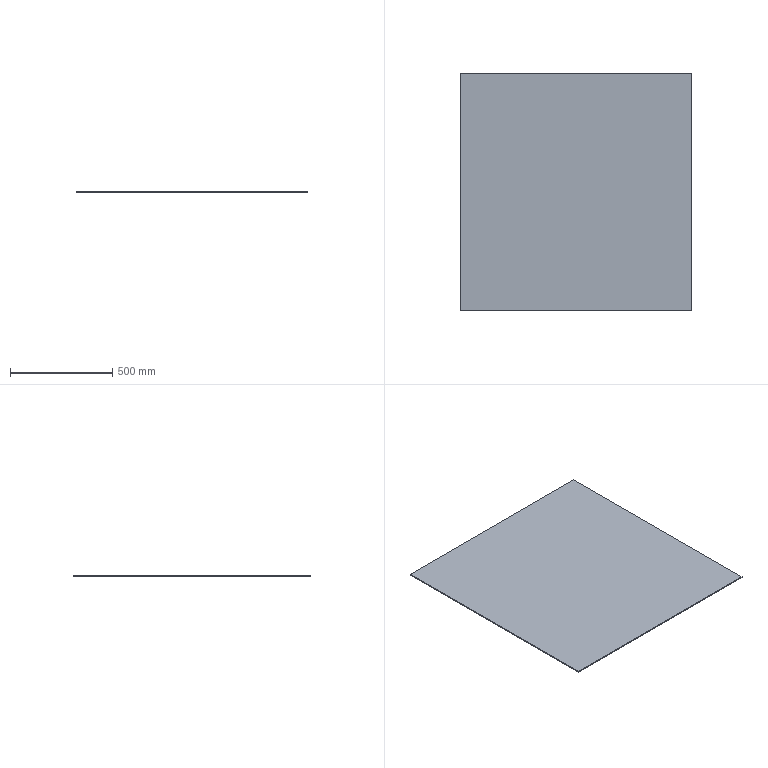Part | 1 solid | 6 faces | box 1135 x 1165 x 5 mm | volume 6611375 mm3 | plane 6
STEP:
#1=CARTESIAN_POINT('',(567.5,-582.5,0.));
#2=VERTEX_POINT('',#1);
#3=CARTESIAN_POINT('',(567.5,582.5,0.));
#4=VERTEX_POINT('',#3);
#5=CARTESIAN_POINT('',(567.5,582.5,0.));
#6=DIRECTION('',(0.,1.,0.));
#7=VECTOR('',#6,1000.);
#8=LINE('',#5,#7);
#9=EDGE_CURVE('',#2,#4,#8,.T.);
#10=ORIENTED_EDGE('',*,*,#9,.T.);
#11=CARTESIAN_POINT('',(567.5,582.5,5.));
#12=VERTEX_POINT('',#11);
#13=CARTESIAN_POINT('',(567.5,582.5,5.));
#14=DIRECTION('',(0.,0.,-1.));
#15=VECTOR('',#14,1000.);
#16=LINE('',#13,#15);
#17=EDGE_CURVE('',#12,#4,#16,.T.);
#18=ORIENTED_EDGE('',*,*,#17,.F.);
#19=CARTESIAN_POINT('',(567.5,-582.5,5.));
#20=VERTEX_POINT('',#19);
#21=CARTESIAN_POINT('',(567.5,582.5,5.));
#22=DIRECTION('',(0.,1.,0.));
#23=VECTOR('',#22,1000.);
#24=LINE('',#21,#23);
#25=EDGE_CURVE('',#20,#12,#24,.T.);
#26=ORIENTED_EDGE('',*,*,#25,.F.);
#27=CARTESIAN_POINT('',(567.5,-582.5,5.));
#28=DIRECTION('',(0.,0.,-1.));
#29=VECTOR('',#28,1000.);
#30=LINE('',#27,#29);
#31=EDGE_CURVE('',#20,#2,#30,.T.);
#32=ORIENTED_EDGE('',*,*,#31,.T.);
#33=EDGE_LOOP('',(#10,#18,#26,#32));
#34=FACE_OUTER_BOUND('',#33,.T.);
#35=CARTESIAN_POINT('',(567.5,582.5,5.));
#36=DIRECTION('',(-1.,0.,0.));
#37=DIRECTION('',(0.,-1.,0.));
#38=AXIS2_PLACEMENT_3D('',#35,#36,#37);
#39=PLANE('',#38);
#40=ADVANCED_FACE('',(#34),#39,.F.);
#41=CARTESIAN_POINT('',(-567.5,582.5,0.));
#42=VERTEX_POINT('',#41);
#43=CARTESIAN_POINT('',(-567.5,582.5,0.));
#44=DIRECTION('',(-1.,0.,0.));
#45=VECTOR('',#44,1000.);
#46=LINE('',#43,#45);
#47=EDGE_CURVE('',#4,#42,#46,.T.);
#48=ORIENTED_EDGE('',*,*,#47,.T.);
#49=CARTESIAN_POINT('',(-567.5,582.5,5.));
#50=VERTEX_POINT('',#49);
#51=CARTESIAN_POINT('',(-567.5,582.5,5.));
#52=DIRECTION('',(0.,0.,-1.));
#53=VECTOR('',#52,1000.);
#54=LINE('',#51,#53);
#55=EDGE_CURVE('',#50,#42,#54,.T.);
#56=ORIENTED_EDGE('',*,*,#55,.F.);
#57=CARTESIAN_POINT('',(-567.5,582.5,5.));
#58=DIRECTION('',(-1.,0.,0.));
#59=VECTOR('',#58,1000.);
#60=LINE('',#57,#59);
#61=EDGE_CURVE('',#12,#50,#60,.T.);
#62=ORIENTED_EDGE('',*,*,#61,.F.);
#63=ORIENTED_EDGE('',*,*,#17,.T.);
#64=EDGE_LOOP('',(#48,#56,#62,#63));
#65=FACE_OUTER_BOUND('',#64,.T.);
#66=CARTESIAN_POINT('',(-567.5,582.5,5.));
#67=DIRECTION('',(0.,-1.,0.));
#68=DIRECTION('',(0.,0.,-1.));
#69=AXIS2_PLACEMENT_3D('',#66,#67,#68);
#70=PLANE('',#69);
#71=ADVANCED_FACE('',(#65),#70,.F.);
#72=CARTESIAN_POINT('',(-567.5,-582.5,0.));
#73=VERTEX_POINT('',#72);
#74=CARTESIAN_POINT('',(-567.5,582.5,0.));
#75=DIRECTION('',(0.,-1.,0.));
#76=VECTOR('',#75,1000.);
#77=LINE('',#74,#76);
#78=EDGE_CURVE('',#42,#73,#77,.T.);
#79=ORIENTED_EDGE('',*,*,#78,.T.);
#80=CARTESIAN_POINT('',(-567.5,-582.5,5.));
#81=VERTEX_POINT('',#80);
#82=CARTESIAN_POINT('',(-567.5,-582.5,5.));
#83=DIRECTION('',(0.,0.,-1.));
#84=VECTOR('',#83,1000.);
#85=LINE('',#82,#84);
#86=EDGE_CURVE('',#81,#73,#85,.T.);
#87=ORIENTED_EDGE('',*,*,#86,.F.);
#88=CARTESIAN_POINT('',(-567.5,582.5,5.));
#89=DIRECTION('',(0.,-1.,0.));
#90=VECTOR('',#89,1000.);
#91=LINE('',#88,#90);
#92=EDGE_CURVE('',#50,#81,#91,.T.);
#93=ORIENTED_EDGE('',*,*,#92,.F.);
#94=ORIENTED_EDGE('',*,*,#55,.T.);
#95=EDGE_LOOP('',(#79,#87,#93,#94));
#96=FACE_OUTER_BOUND('',#95,.T.);
#97=CARTESIAN_POINT('',(-567.5,582.5,5.));
#98=DIRECTION('',(1.,0.,0.));
#99=DIRECTION('',(0.,1.,0.));
#100=AXIS2_PLACEMENT_3D('',#97,#98,#99);
#101=PLANE('',#100);
#102=ADVANCED_FACE('',(#96),#101,.F.);
#103=CARTESIAN_POINT('',(-567.5,-582.5,0.));
#104=DIRECTION('',(1.,0.,0.));
#105=VECTOR('',#104,1000.);
#106=LINE('',#103,#105);
#107=EDGE_CURVE('',#73,#2,#106,.T.);
#108=ORIENTED_EDGE('',*,*,#107,.T.);
#109=ORIENTED_EDGE('',*,*,#31,.F.);
#110=CARTESIAN_POINT('',(-567.5,-582.5,5.));
#111=DIRECTION('',(1.,0.,0.));
#112=VECTOR('',#111,1000.);
#113=LINE('',#110,#112);
#114=EDGE_CURVE('',#81,#20,#113,.T.);
#115=ORIENTED_EDGE('',*,*,#114,.F.);
#116=ORIENTED_EDGE('',*,*,#86,.T.);
#117=EDGE_LOOP('',(#108,#109,#115,#116));
#118=FACE_OUTER_BOUND('',#117,.T.);
#119=CARTESIAN_POINT('',(-567.5,-582.5,5.));
#120=DIRECTION('',(0.,1.,0.));
#121=DIRECTION('',(0.,0.,1.));
#122=AXIS2_PLACEMENT_3D('',#119,#120,#121);
#123=PLANE('',#122);
#124=ADVANCED_FACE('',(#118),#123,.F.);
#125=ORIENTED_EDGE('',*,*,#25,.T.);
#126=ORIENTED_EDGE('',*,*,#61,.T.);
#127=ORIENTED_EDGE('',*,*,#92,.T.);
#128=ORIENTED_EDGE('',*,*,#114,.T.);
#129=EDGE_LOOP('',(#125,#126,#127,#128));
#130=FACE_OUTER_BOUND('',#129,.T.);
#131=CARTESIAN_POINT('',(0.,0.,5.));
#132=DIRECTION('',(0.,0.,1.));
#133=DIRECTION('',(1.,0.,0.));
#134=AXIS2_PLACEMENT_3D('',#131,#132,#133);
#135=PLANE('',#134);
#136=ADVANCED_FACE('',(#130),#135,.T.);
#137=ORIENTED_EDGE('',*,*,#9,.F.);
#138=ORIENTED_EDGE('',*,*,#107,.F.);
#139=ORIENTED_EDGE('',*,*,#78,.F.);
#140=ORIENTED_EDGE('',*,*,#47,.F.);
#141=EDGE_LOOP('',(#137,#138,#139,#140));
#142=FACE_OUTER_BOUND('',#141,.T.);
#143=CARTESIAN_POINT('',(0.,0.,0.));
#144=DIRECTION('',(0.,0.,1.));
#145=DIRECTION('',(1.,0.,0.));
#146=AXIS2_PLACEMENT_3D('',#143,#144,#145);
#147=PLANE('',#146);
#148=ADVANCED_FACE('',(#142),#147,.F.);
#149=CLOSED_SHELL('',(#40,#71,#102,#124,#136,#148));
#150=MANIFOLD_SOLID_BREP('',#149);
#151=CARTESIAN_POINT('',(0.,0.,0.));
#152=DIRECTION('',(0.,0.,1.));
#153=DIRECTION('',(1.,0.,0.));
#154=AXIS2_PLACEMENT_3D('',#151,#152,#153);
#155=(LENGTH_UNIT()NAMED_UNIT(*)SI_UNIT(.MILLI.,.METRE.));
#156=UNCERTAINTY_MEASURE_WITH_UNIT(LENGTH_MEASURE(0.00001),#155,'','');
#157=(NAMED_UNIT(*)PLANE_ANGLE_UNIT()SI_UNIT($,.RADIAN.));
#158=(NAMED_UNIT(*)SI_UNIT($,.STERADIAN.)SOLID_ANGLE_UNIT());
#159=(GEOMETRIC_REPRESENTATION_CONTEXT(3)GLOBAL_UNCERTAINTY_ASSIGNED_CONTEXT((#156))GLOBAL_UNIT_ASSIGNED_CONTEXT((#155,#157,#158))REPRESENTATION_CONTEXT('',''));
#160=ADVANCED_BREP_SHAPE_REPRESENTATION('',(#150,#154),#159);